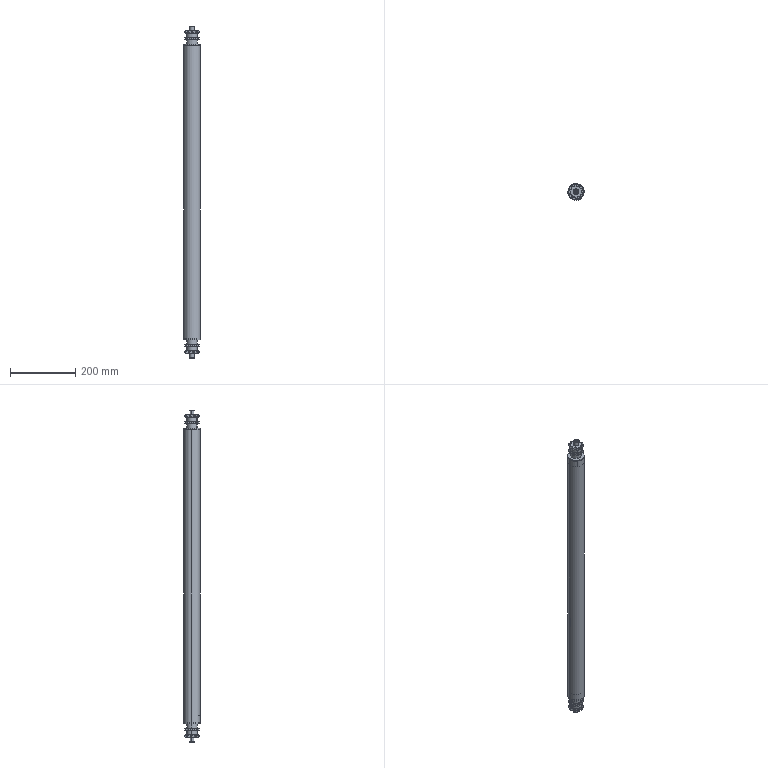Part | SolidWorks | 4 solids | 388 faces | box 50 x 50 x 1020 mm | volume 482112 mm3 | plane 178 | cylinder 114 | cone 96 | commonest cylinder face diameters 46 x44 7.92 x40 32 x8 47.6 x6 50 x6 6.8 x4